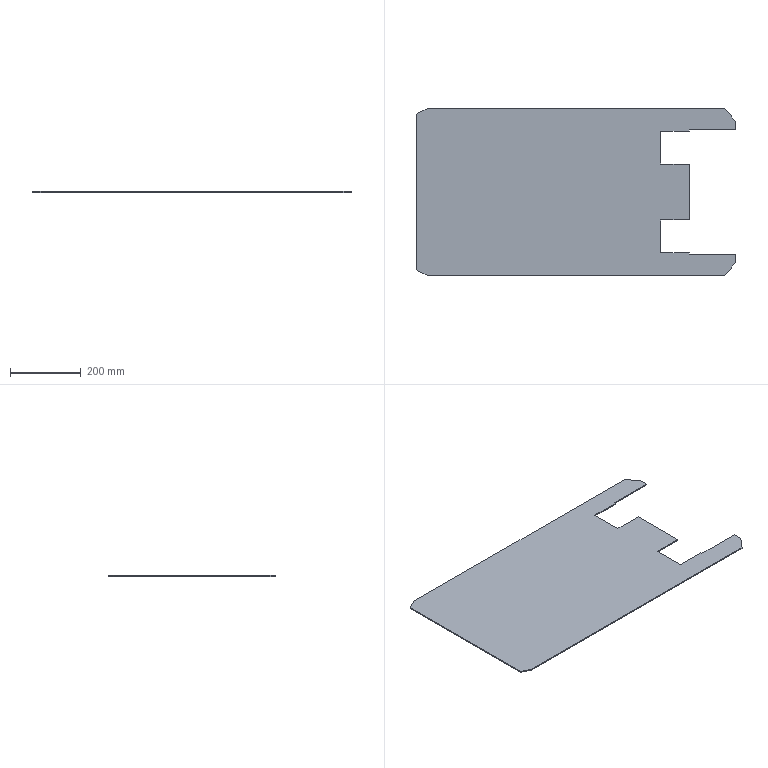Part | SolidWorks | features Extrusion 1, ICE 1 | 1 solid | 22 faces | box 900 x 470 x 3 mm | volume 1083288 mm3 | plane 22
STEP:
#1=CARTESIAN_POINT('',(150.,171.,-1.5));
#2=VERTEX_POINT('',#1);
#3=CARTESIAN_POINT('',(150.,171.,1.5));
#4=VERTEX_POINT('',#3);
#5=CARTESIAN_POINT('',(150.,171.,-1.5));
#6=DIRECTION('',(0.,0.,1.));
#7=VECTOR('',#6,1000.);
#8=LINE('',#5,#7);
#9=EDGE_CURVE('',#2,#4,#8,.T.);
#10=ORIENTED_EDGE('',*,*,#9,.F.);
#11=CARTESIAN_POINT('',(150.,175.,-1.5));
#12=VERTEX_POINT('',#11);
#13=CARTESIAN_POINT('',(150.,-175.,-1.5));
#14=DIRECTION('',(0.,1.,0.));
#15=VECTOR('',#14,1000.);
#16=LINE('',#13,#15);
#17=EDGE_CURVE('',#2,#12,#16,.T.);
#18=ORIENTED_EDGE('',*,*,#17,.T.);
#19=CARTESIAN_POINT('',(150.,175.,1.5));
#20=VERTEX_POINT('',#19);
#21=CARTESIAN_POINT('',(150.,175.,-1.5));
#22=DIRECTION('',(0.,0.,1.));
#23=VECTOR('',#22,1000.);
#24=LINE('',#21,#23);
#25=EDGE_CURVE('',#12,#20,#24,.T.);
#26=ORIENTED_EDGE('',*,*,#25,.T.);
#27=CARTESIAN_POINT('',(150.,-175.,1.5));
#28=DIRECTION('',(0.,1.,0.));
#29=VECTOR('',#28,1000.);
#30=LINE('',#27,#29);
#31=EDGE_CURVE('',#4,#20,#30,.T.);
#32=ORIENTED_EDGE('',*,*,#31,.F.);
#33=EDGE_LOOP('',(#10,#18,#26,#32));
#34=FACE_OUTER_BOUND('',#33,.T.);
#35=CARTESIAN_POINT('',(150.,-175.,-1.5));
#36=DIRECTION('',(1.,0.,0.));
#37=DIRECTION('',(0.,0.,-1.));
#38=AXIS2_PLACEMENT_3D('',#35,#36,#37);
#39=PLANE('',#38);
#40=ADVANCED_FACE('',(#34),#39,.T.);
#41=CARTESIAN_POINT('',(150.,79.,1.5));
#42=VERTEX_POINT('',#41);
#43=CARTESIAN_POINT('',(150.,79.,-1.5));
#44=VERTEX_POINT('',#43);
#45=CARTESIAN_POINT('',(150.,79.,-1.5));
#46=DIRECTION('',(0.,0.,-1.));
#47=VECTOR('',#46,1000.);
#48=LINE('',#45,#47);
#49=EDGE_CURVE('',#42,#44,#48,.T.);
#50=ORIENTED_EDGE('',*,*,#49,.F.);
#51=CARTESIAN_POINT('',(150.,-79.,1.5));
#52=VERTEX_POINT('',#51);
#53=CARTESIAN_POINT('',(150.,-175.,1.5));
#54=DIRECTION('',(0.,1.,0.));
#55=VECTOR('',#54,1000.);
#56=LINE('',#53,#55);
#57=EDGE_CURVE('',#52,#42,#56,.T.);
#58=ORIENTED_EDGE('',*,*,#57,.F.);
#59=CARTESIAN_POINT('',(150.,-79.,-1.5));
#60=VERTEX_POINT('',#59);
#61=CARTESIAN_POINT('',(150.,-79.,-1.5));
#62=DIRECTION('',(0.,0.,1.));
#63=VECTOR('',#62,1000.);
#64=LINE('',#61,#63);
#65=EDGE_CURVE('',#60,#52,#64,.T.);
#66=ORIENTED_EDGE('',*,*,#65,.F.);
#67=CARTESIAN_POINT('',(150.,-175.,-1.5));
#68=DIRECTION('',(0.,1.,0.));
#69=VECTOR('',#68,1000.);
#70=LINE('',#67,#69);
#71=EDGE_CURVE('',#60,#44,#70,.T.);
#72=ORIENTED_EDGE('',*,*,#71,.T.);
#73=EDGE_LOOP('',(#50,#58,#66,#72));
#74=FACE_OUTER_BOUND('',#73,.T.);
#75=CARTESIAN_POINT('',(150.,-175.,-1.5));
#76=DIRECTION('',(1.,0.,0.));
#77=DIRECTION('',(0.,0.,-1.));
#78=AXIS2_PLACEMENT_3D('',#75,#76,#77);
#79=PLANE('',#78);
#80=ADVANCED_FACE('',(#74),#79,.T.);
#81=CARTESIAN_POINT('',(-620.,220.,1.5));
#82=VERTEX_POINT('',#81);
#83=CARTESIAN_POINT('',(-620.,-220.,1.5));
#84=VERTEX_POINT('',#83);
#85=CARTESIAN_POINT('',(-620.,220.,1.5));
#86=DIRECTION('',(0.,-1.,0.));
#87=VECTOR('',#86,1000.);
#88=LINE('',#85,#87);
#89=EDGE_CURVE('',#82,#84,#88,.T.);
#90=ORIENTED_EDGE('',*,*,#89,.F.);
#91=CARTESIAN_POINT('',(-620.,220.,-1.5));
#92=VERTEX_POINT('',#91);
#93=CARTESIAN_POINT('',(-620.,220.,-1.5));
#94=DIRECTION('',(0.,0.,1.));
#95=VECTOR('',#94,1000.);
#96=LINE('',#93,#95);
#97=EDGE_CURVE('',#92,#82,#96,.T.);
#98=ORIENTED_EDGE('',*,*,#97,.F.);
#99=CARTESIAN_POINT('',(-620.,-220.,-1.5));
#100=VERTEX_POINT('',#99);
#101=CARTESIAN_POINT('',(-620.,220.,-1.5));
#102=DIRECTION('',(0.,-1.,0.));
#103=VECTOR('',#102,1000.);
#104=LINE('',#101,#103);
#105=EDGE_CURVE('',#92,#100,#104,.T.);
#106=ORIENTED_EDGE('',*,*,#105,.T.);
#107=CARTESIAN_POINT('',(-620.,-220.,-1.5));
#108=DIRECTION('',(0.,0.,1.));
#109=VECTOR('',#108,1000.);
#110=LINE('',#107,#109);
#111=EDGE_CURVE('',#100,#84,#110,.T.);
#112=ORIENTED_EDGE('',*,*,#111,.T.);
#113=EDGE_LOOP('',(#90,#98,#106,#112));
#114=FACE_OUTER_BOUND('',#113,.T.);
#115=CARTESIAN_POINT('',(-620.,220.,-1.5));
#116=DIRECTION('',(-1.,0.,0.));
#117=DIRECTION('',(0.,0.,1.));
#118=AXIS2_PLACEMENT_3D('',#115,#116,#117);
#119=PLANE('',#118);
#120=ADVANCED_FACE('',(#114),#119,.T.);
#121=CARTESIAN_POINT('',(-590.,235.,1.5));
#122=VERTEX_POINT('',#121);
#123=CARTESIAN_POINT('',(-590.,235.,1.5));
#124=DIRECTION('',(-0.8944,-0.4472,0.));
#125=VECTOR('',#124,1000.);
#126=LINE('',#123,#125);
#127=EDGE_CURVE('',#122,#82,#126,.T.);
#128=ORIENTED_EDGE('',*,*,#127,.F.);
#129=CARTESIAN_POINT('',(-590.,235.,-1.5));
#130=VERTEX_POINT('',#129);
#131=CARTESIAN_POINT('',(-590.,235.,-1.5));
#132=DIRECTION('',(0.,0.,1.));
#133=VECTOR('',#132,1000.);
#134=LINE('',#131,#133);
#135=EDGE_CURVE('',#130,#122,#134,.T.);
#136=ORIENTED_EDGE('',*,*,#135,.F.);
#137=CARTESIAN_POINT('',(-590.,235.,-1.5));
#138=DIRECTION('',(-0.8944,-0.4472,0.));
#139=VECTOR('',#138,1000.);
#140=LINE('',#137,#139);
#141=EDGE_CURVE('',#130,#92,#140,.T.);
#142=ORIENTED_EDGE('',*,*,#141,.T.);
#143=ORIENTED_EDGE('',*,*,#97,.T.);
#144=EDGE_LOOP('',(#128,#136,#142,#143));
#145=FACE_OUTER_BOUND('',#144,.T.);
#146=CARTESIAN_POINT('',(-590.,235.,-1.5));
#147=DIRECTION('',(-0.4472,0.8944,0.));
#148=DIRECTION('',(-0.8944,-0.4472,0.));
#149=AXIS2_PLACEMENT_3D('',#146,#147,#148);
#150=PLANE('',#149);
#151=ADVANCED_FACE('',(#145),#150,.T.);
#152=CARTESIAN_POINT('',(250.,235.,1.5));
#153=VERTEX_POINT('',#152);
#154=CARTESIAN_POINT('',(250.,235.,1.5));
#155=DIRECTION('',(-1.,0.,0.));
#156=VECTOR('',#155,1000.);
#157=LINE('',#154,#156);
#158=EDGE_CURVE('',#153,#122,#157,.T.);
#159=ORIENTED_EDGE('',*,*,#158,.F.);
#160=CARTESIAN_POINT('',(250.,235.,-1.5));
#161=VERTEX_POINT('',#160);
#162=CARTESIAN_POINT('',(250.,235.,-1.5));
#163=DIRECTION('',(0.,0.,1.));
#164=VECTOR('',#163,1000.);
#165=LINE('',#162,#164);
#166=EDGE_CURVE('',#161,#153,#165,.T.);
#167=ORIENTED_EDGE('',*,*,#166,.F.);
#168=CARTESIAN_POINT('',(250.,235.,-1.5));
#169=DIRECTION('',(-1.,0.,0.));
#170=VECTOR('',#169,1000.);
#171=LINE('',#168,#170);
#172=EDGE_CURVE('',#161,#130,#171,.T.);
#173=ORIENTED_EDGE('',*,*,#172,.T.);
#174=ORIENTED_EDGE('',*,*,#135,.T.);
#175=EDGE_LOOP('',(#159,#167,#173,#174));
#176=FACE_OUTER_BOUND('',#175,.T.);
#177=CARTESIAN_POINT('',(250.,235.,-1.5));
#178=DIRECTION('',(0.,1.,0.));
#179=DIRECTION('',(0.,0.,1.));
#180=AXIS2_PLACEMENT_3D('',#177,#178,#179);
#181=PLANE('',#180);
#182=ADVANCED_FACE('',(#176),#181,.T.);
#183=CARTESIAN_POINT('',(280.,200.,1.5));
#184=VERTEX_POINT('',#183);
#185=CARTESIAN_POINT('',(280.,200.,1.5));
#186=DIRECTION('',(-0.6508,0.7593,0.));
#187=VECTOR('',#186,1000.);
#188=LINE('',#185,#187);
#189=EDGE_CURVE('',#184,#153,#188,.T.);
#190=ORIENTED_EDGE('',*,*,#189,.F.);
#191=CARTESIAN_POINT('',(280.,200.,-1.5));
#192=VERTEX_POINT('',#191);
#193=CARTESIAN_POINT('',(280.,200.,-1.5));
#194=DIRECTION('',(0.,0.,1.));
#195=VECTOR('',#194,1000.);
#196=LINE('',#193,#195);
#197=EDGE_CURVE('',#192,#184,#196,.T.);
#198=ORIENTED_EDGE('',*,*,#197,.F.);
#199=CARTESIAN_POINT('',(280.,200.,-1.5));
#200=DIRECTION('',(-0.6508,0.7593,0.));
#201=VECTOR('',#200,1000.);
#202=LINE('',#199,#201);
#203=EDGE_CURVE('',#192,#161,#202,.T.);
#204=ORIENTED_EDGE('',*,*,#203,.T.);
#205=ORIENTED_EDGE('',*,*,#166,.T.);
#206=EDGE_LOOP('',(#190,#198,#204,#205));
#207=FACE_OUTER_BOUND('',#206,.T.);
#208=CARTESIAN_POINT('',(280.,200.,-1.5));
#209=DIRECTION('',(0.7593,0.6508,0.));
#210=DIRECTION('',(-0.6508,0.7593,0.));
#211=AXIS2_PLACEMENT_3D('',#208,#209,#210);
#212=PLANE('',#211);
#213=ADVANCED_FACE('',(#207),#212,.T.);
#214=CARTESIAN_POINT('',(280.,175.,1.5));
#215=VERTEX_POINT('',#214);
#216=CARTESIAN_POINT('',(280.,175.,1.5));
#217=DIRECTION('',(0.,1.,0.));
#218=VECTOR('',#217,1000.);
#219=LINE('',#216,#218);
#220=EDGE_CURVE('',#215,#184,#219,.T.);
#221=ORIENTED_EDGE('',*,*,#220,.F.);
#222=CARTESIAN_POINT('',(280.,175.,-1.5));
#223=VERTEX_POINT('',#222);
#224=CARTESIAN_POINT('',(280.,175.,-1.5));
#225=DIRECTION('',(0.,0.,1.));
#226=VECTOR('',#225,1000.);
#227=LINE('',#224,#226);
#228=EDGE_CURVE('',#223,#215,#227,.T.);
#229=ORIENTED_EDGE('',*,*,#228,.F.);
#230=CARTESIAN_POINT('',(280.,175.,-1.5));
#231=DIRECTION('',(0.,1.,0.));
#232=VECTOR('',#231,1000.);
#233=LINE('',#230,#232);
#234=EDGE_CURVE('',#223,#192,#233,.T.);
#235=ORIENTED_EDGE('',*,*,#234,.T.);
#236=ORIENTED_EDGE('',*,*,#197,.T.);
#237=EDGE_LOOP('',(#221,#229,#235,#236));
#238=FACE_OUTER_BOUND('',#237,.T.);
#239=CARTESIAN_POINT('',(280.,175.,-1.5));
#240=DIRECTION('',(1.,0.,0.));
#241=DIRECTION('',(0.,0.,-1.));
#242=AXIS2_PLACEMENT_3D('',#239,#240,#241);
#243=PLANE('',#242);
#244=ADVANCED_FACE('',(#238),#243,.T.);
#245=CARTESIAN_POINT('',(150.,175.,1.5));
#246=DIRECTION('',(1.,0.,0.));
#247=VECTOR('',#246,1000.);
#248=LINE('',#245,#247);
#249=EDGE_CURVE('',#20,#215,#248,.T.);
#250=ORIENTED_EDGE('',*,*,#249,.F.);
#251=ORIENTED_EDGE('',*,*,#25,.F.);
#252=CARTESIAN_POINT('',(150.,175.,-1.5));
#253=DIRECTION('',(1.,0.,0.));
#254=VECTOR('',#253,1000.);
#255=LINE('',#252,#254);
#256=EDGE_CURVE('',#12,#223,#255,.T.);
#257=ORIENTED_EDGE('',*,*,#256,.T.);
#258=ORIENTED_EDGE('',*,*,#228,.T.);
#259=EDGE_LOOP('',(#250,#251,#257,#258));
#260=FACE_OUTER_BOUND('',#259,.T.);
#261=CARTESIAN_POINT('',(150.,175.,-1.5));
#262=DIRECTION('',(0.,-1.,0.));
#263=DIRECTION('',(0.,0.,-1.));
#264=AXIS2_PLACEMENT_3D('',#261,#262,#263);
#265=PLANE('',#264);
#266=ADVANCED_FACE('',(#260),#265,.T.);
#267=CARTESIAN_POINT('',(150.,-171.,1.5));
#268=VERTEX_POINT('',#267);
#269=CARTESIAN_POINT('',(150.,-171.,-1.5));
#270=VERTEX_POINT('',#269);
#271=CARTESIAN_POINT('',(150.,-171.,-1.5));
#272=DIRECTION('',(0.,0.,-1.));
#273=VECTOR('',#272,1000.);
#274=LINE('',#271,#273);
#275=EDGE_CURVE('',#268,#270,#274,.T.);
#276=ORIENTED_EDGE('',*,*,#275,.F.);
#277=CARTESIAN_POINT('',(150.,-175.,1.5));
#278=VERTEX_POINT('',#277);
#279=CARTESIAN_POINT('',(150.,-175.,1.5));
#280=DIRECTION('',(0.,1.,0.));
#281=VECTOR('',#280,1000.);
#282=LINE('',#279,#281);
#283=EDGE_CURVE('',#278,#268,#282,.T.);
#284=ORIENTED_EDGE('',*,*,#283,.F.);
#285=CARTESIAN_POINT('',(150.,-175.,-1.5));
#286=VERTEX_POINT('',#285);
#287=CARTESIAN_POINT('',(150.,-175.,-1.5));
#288=DIRECTION('',(0.,0.,1.));
#289=VECTOR('',#288,1000.);
#290=LINE('',#287,#289);
#291=EDGE_CURVE('',#286,#278,#290,.T.);
#292=ORIENTED_EDGE('',*,*,#291,.F.);
#293=CARTESIAN_POINT('',(150.,-175.,-1.5));
#294=DIRECTION('',(0.,1.,0.));
#295=VECTOR('',#294,1000.);
#296=LINE('',#293,#295);
#297=EDGE_CURVE('',#286,#270,#296,.T.);
#298=ORIENTED_EDGE('',*,*,#297,.T.);
#299=EDGE_LOOP('',(#276,#284,#292,#298));
#300=FACE_OUTER_BOUND('',#299,.T.);
#301=CARTESIAN_POINT('',(150.,-175.,-1.5));
#302=DIRECTION('',(1.,0.,0.));
#303=DIRECTION('',(0.,0.,-1.));
#304=AXIS2_PLACEMENT_3D('',#301,#302,#303);
#305=PLANE('',#304);
#306=ADVANCED_FACE('',(#300),#305,.T.);
#307=CARTESIAN_POINT('',(280.,-175.,1.5));
#308=VERTEX_POINT('',#307);
#309=CARTESIAN_POINT('',(280.,-175.,1.5));
#310=DIRECTION('',(-1.,0.,0.));
#311=VECTOR('',#310,1000.);
#312=LINE('',#309,#311);
#313=EDGE_CURVE('',#308,#278,#312,.T.);
#314=ORIENTED_EDGE('',*,*,#313,.F.);
#315=CARTESIAN_POINT('',(280.,-175.,-1.5));
#316=VERTEX_POINT('',#315);
#317=CARTESIAN_POINT('',(280.,-175.,-1.5));
#318=DIRECTION('',(0.,0.,1.));
#319=VECTOR('',#318,1000.);
#320=LINE('',#317,#319);
#321=EDGE_CURVE('',#316,#308,#320,.T.);
#322=ORIENTED_EDGE('',*,*,#321,.F.);
#323=CARTESIAN_POINT('',(280.,-175.,-1.5));
#324=DIRECTION('',(-1.,0.,0.));
#325=VECTOR('',#324,1000.);
#326=LINE('',#323,#325);
#327=EDGE_CURVE('',#316,#286,#326,.T.);
#328=ORIENTED_EDGE('',*,*,#327,.T.);
#329=ORIENTED_EDGE('',*,*,#291,.T.);
#330=EDGE_LOOP('',(#314,#322,#328,#329));
#331=FACE_OUTER_BOUND('',#330,.T.);
#332=CARTESIAN_POINT('',(280.,-175.,-1.5));
#333=DIRECTION('',(0.,1.,0.));
#334=DIRECTION('',(0.,0.,1.));
#335=AXIS2_PLACEMENT_3D('',#332,#333,#334);
#336=PLANE('',#335);
#337=ADVANCED_FACE('',(#331),#336,.T.);
#338=CARTESIAN_POINT('',(280.,-200.,1.5));
#339=VERTEX_POINT('',#338);
#340=CARTESIAN_POINT('',(280.,-200.,1.5));
#341=DIRECTION('',(0.,1.,0.));
#342=VECTOR('',#341,1000.);
#343=LINE('',#340,#342);
#344=EDGE_CURVE('',#339,#308,#343,.T.);
#345=ORIENTED_EDGE('',*,*,#344,.F.);
#346=CARTESIAN_POINT('',(280.,-200.,-1.5));
#347=VERTEX_POINT('',#346);
#348=CARTESIAN_POINT('',(280.,-200.,-1.5));
#349=DIRECTION('',(0.,0.,1.));
#350=VECTOR('',#349,1000.);
#351=LINE('',#348,#350);
#352=EDGE_CURVE('',#347,#339,#351,.T.);
#353=ORIENTED_EDGE('',*,*,#352,.F.);
#354=CARTESIAN_POINT('',(280.,-200.,-1.5));
#355=DIRECTION('',(0.,1.,0.));
#356=VECTOR('',#355,1000.);
#357=LINE('',#354,#356);
#358=EDGE_CURVE('',#347,#316,#357,.T.);
#359=ORIENTED_EDGE('',*,*,#358,.T.);
#360=ORIENTED_EDGE('',*,*,#321,.T.);
#361=EDGE_LOOP('',(#345,#353,#359,#360));
#362=FACE_OUTER_BOUND('',#361,.T.);
#363=CARTESIAN_POINT('',(280.,-200.,-1.5));
#364=DIRECTION('',(1.,0.,0.));
#365=DIRECTION('',(0.,0.,-1.));
#366=AXIS2_PLACEMENT_3D('',#363,#364,#365);
#367=PLANE('',#366);
#368=ADVANCED_FACE('',(#362),#367,.T.);
#369=CARTESIAN_POINT('',(250.,-235.,1.5));
#370=VERTEX_POINT('',#369);
#371=CARTESIAN_POINT('',(250.,-235.,1.5));
#372=DIRECTION('',(0.6508,0.7593,0.));
#373=VECTOR('',#372,1000.);
#374=LINE('',#371,#373);
#375=EDGE_CURVE('',#370,#339,#374,.T.);
#376=ORIENTED_EDGE('',*,*,#375,.F.);
#377=CARTESIAN_POINT('',(250.,-235.,-1.5));
#378=VERTEX_POINT('',#377);
#379=CARTESIAN_POINT('',(250.,-235.,-1.5));
#380=DIRECTION('',(0.,0.,1.));
#381=VECTOR('',#380,1000.);
#382=LINE('',#379,#381);
#383=EDGE_CURVE('',#378,#370,#382,.T.);
#384=ORIENTED_EDGE('',*,*,#383,.F.);
#385=CARTESIAN_POINT('',(250.,-235.,-1.5));
#386=DIRECTION('',(0.6508,0.7593,0.));
#387=VECTOR('',#386,1000.);
#388=LINE('',#385,#387);
#389=EDGE_CURVE('',#378,#347,#388,.T.);
#390=ORIENTED_EDGE('',*,*,#389,.T.);
#391=ORIENTED_EDGE('',*,*,#352,.T.);
#392=EDGE_LOOP('',(#376,#384,#390,#391));
#393=FACE_OUTER_BOUND('',#392,.T.);
#394=CARTESIAN_POINT('',(250.,-235.,-1.5));
#395=DIRECTION('',(0.7593,-0.6508,0.));
#396=DIRECTION('',(0.6508,0.7593,0.));
#397=AXIS2_PLACEMENT_3D('',#394,#395,#396);
#398=PLANE('',#397);
#399=ADVANCED_FACE('',(#393),#398,.T.);
#400=CARTESIAN_POINT('',(-590.,-235.,1.5));
#401=VERTEX_POINT('',#400);
#402=CARTESIAN_POINT('',(-590.,-235.,1.5));
#403=DIRECTION('',(1.,0.,0.));
#404=VECTOR('',#403,1000.);
#405=LINE('',#402,#404);
#406=EDGE_CURVE('',#401,#370,#405,.T.);
#407=ORIENTED_EDGE('',*,*,#406,.F.);
#408=CARTESIAN_POINT('',(-590.,-235.,-1.5));
#409=VERTEX_POINT('',#408);
#410=CARTESIAN_POINT('',(-590.,-235.,-1.5));
#411=DIRECTION('',(0.,0.,1.));
#412=VECTOR('',#411,1000.);
#413=LINE('',#410,#412);
#414=EDGE_CURVE('',#409,#401,#413,.T.);
#415=ORIENTED_EDGE('',*,*,#414,.F.);
#416=CARTESIAN_POINT('',(-590.,-235.,-1.5));
#417=DIRECTION('',(1.,0.,0.));
#418=VECTOR('',#417,1000.);
#419=LINE('',#416,#418);
#420=EDGE_CURVE('',#409,#378,#419,.T.);
#421=ORIENTED_EDGE('',*,*,#420,.T.);
#422=ORIENTED_EDGE('',*,*,#383,.T.);
#423=EDGE_LOOP('',(#407,#415,#421,#422));
#424=FACE_OUTER_BOUND('',#423,.T.);
#425=CARTESIAN_POINT('',(-590.,-235.,-1.5));
#426=DIRECTION('',(0.,-1.,0.));
#427=DIRECTION('',(0.,0.,-1.));
#428=AXIS2_PLACEMENT_3D('',#425,#426,#427);
#429=PLANE('',#428);
#430=ADVANCED_FACE('',(#424),#429,.T.);
#431=CARTESIAN_POINT('',(-620.,-220.,1.5));
#432=DIRECTION('',(0.8944,-0.4472,0.));
#433=VECTOR('',#432,1000.);
#434=LINE('',#431,#433);
#435=EDGE_CURVE('',#84,#401,#434,.T.);
#436=ORIENTED_EDGE('',*,*,#435,.F.);
#437=ORIENTED_EDGE('',*,*,#111,.F.);
#438=CARTESIAN_POINT('',(-620.,-220.,-1.5));
#439=DIRECTION('',(0.8944,-0.4472,0.));
#440=VECTOR('',#439,1000.);
#441=LINE('',#438,#440);
#442=EDGE_CURVE('',#100,#409,#441,.T.);
#443=ORIENTED_EDGE('',*,*,#442,.T.);
#444=ORIENTED_EDGE('',*,*,#414,.T.);
#445=EDGE_LOOP('',(#436,#437,#443,#444));
#446=FACE_OUTER_BOUND('',#445,.T.);
#447=CARTESIAN_POINT('',(-620.,-220.,-1.5));
#448=DIRECTION('',(-0.4472,-0.8944,0.));
#449=DIRECTION('',(0.8944,-0.4472,0.));
#450=AXIS2_PLACEMENT_3D('',#447,#448,#449);
#451=PLANE('',#450);
#452=ADVANCED_FACE('',(#446),#451,.T.);
#453=ORIENTED_EDGE('',*,*,#17,.F.);
#454=CARTESIAN_POINT('',(69.,171.,-1.5));
#455=VERTEX_POINT('',#454);
#456=CARTESIAN_POINT('',(0.,171.,-1.5));
#457=DIRECTION('',(-1.,0.,0.));
#458=VECTOR('',#457,1000.);
#459=LINE('',#456,#458);
#460=EDGE_CURVE('',#2,#455,#459,.T.);
#461=ORIENTED_EDGE('',*,*,#460,.T.);
#462=CARTESIAN_POINT('',(69.,79.,-1.5));
#463=VERTEX_POINT('',#462);
#464=CARTESIAN_POINT('',(69.,0.,-1.5));
#465=DIRECTION('',(0.,-1.,0.));
#466=VECTOR('',#465,1000.);
#467=LINE('',#464,#466);
#468=EDGE_CURVE('',#455,#463,#467,.T.);
#469=ORIENTED_EDGE('',*,*,#468,.T.);
#470=CARTESIAN_POINT('',(0.,79.,-1.5));
#471=DIRECTION('',(1.,0.,0.));
#472=VECTOR('',#471,1000.);
#473=LINE('',#470,#472);
#474=EDGE_CURVE('',#463,#44,#473,.T.);
#475=ORIENTED_EDGE('',*,*,#474,.T.);
#476=ORIENTED_EDGE('',*,*,#71,.F.);
#477=CARTESIAN_POINT('',(69.,-79.,-1.5));
#478=VERTEX_POINT('',#477);
#479=CARTESIAN_POINT('',(0.,-79.,-1.5));
#480=DIRECTION('',(-1.,0.,0.));
#481=VECTOR('',#480,1000.);
#482=LINE('',#479,#481);
#483=EDGE_CURVE('',#60,#478,#482,.T.);
#484=ORIENTED_EDGE('',*,*,#483,.T.);
#485=CARTESIAN_POINT('',(69.,-171.,-1.5));
#486=VERTEX_POINT('',#485);
#487=CARTESIAN_POINT('',(69.,0.,-1.5));
#488=DIRECTION('',(0.,-1.,0.));
#489=VECTOR('',#488,1000.);
#490=LINE('',#487,#489);
#491=EDGE_CURVE('',#478,#486,#490,.T.);
#492=ORIENTED_EDGE('',*,*,#491,.T.);
#493=CARTESIAN_POINT('',(0.,-171.,-1.5));
#494=DIRECTION('',(1.,0.,0.));
#495=VECTOR('',#494,1000.);
#496=LINE('',#493,#495);
#497=EDGE_CURVE('',#486,#270,#496,.T.);
#498=ORIENTED_EDGE('',*,*,#497,.T.);
#499=ORIENTED_EDGE('',*,*,#297,.F.);
#500=ORIENTED_EDGE('',*,*,#327,.F.);
#501=ORIENTED_EDGE('',*,*,#358,.F.);
#502=ORIENTED_EDGE('',*,*,#389,.F.);
#503=ORIENTED_EDGE('',*,*,#420,.F.);
#504=ORIENTED_EDGE('',*,*,#442,.F.);
#505=ORIENTED_EDGE('',*,*,#105,.F.);
#506=ORIENTED_EDGE('',*,*,#141,.F.);
#507=ORIENTED_EDGE('',*,*,#172,.F.);
#508=ORIENTED_EDGE('',*,*,#203,.F.);
#509=ORIENTED_EDGE('',*,*,#234,.F.);
#510=ORIENTED_EDGE('',*,*,#256,.F.);
#511=EDGE_LOOP('',(#453,#461,#469,#475,#476,#484,#492,#498,#499,#500,#501,#502,#503,#504,#505,#506,#507,#508,#509,#510));
#512=FACE_OUTER_BOUND('',#511,.T.);
#513=CARTESIAN_POINT('',(0.,0.,-1.5));
#514=DIRECTION('',(0.,0.,1.));
#515=DIRECTION('',(1.,0.,0.));
#516=AXIS2_PLACEMENT_3D('',#513,#514,#515);
#517=PLANE('',#516);
#518=ADVANCED_FACE('',(#512),#517,.F.);
#519=CARTESIAN_POINT('',(69.,171.,1.5));
#520=VERTEX_POINT('',#519);
#521=CARTESIAN_POINT('',(0.,171.,1.5));
#522=DIRECTION('',(-1.,0.,0.));
#523=VECTOR('',#522,1000.);
#524=LINE('',#521,#523);
#525=EDGE_CURVE('',#4,#520,#524,.T.);
#526=ORIENTED_EDGE('',*,*,#525,.F.);
#527=ORIENTED_EDGE('',*,*,#31,.T.);
#528=ORIENTED_EDGE('',*,*,#249,.T.);
#529=ORIENTED_EDGE('',*,*,#220,.T.);
#530=ORIENTED_EDGE('',*,*,#189,.T.);
#531=ORIENTED_EDGE('',*,*,#158,.T.);
#532=ORIENTED_EDGE('',*,*,#127,.T.);
#533=ORIENTED_EDGE('',*,*,#89,.T.);
#534=ORIENTED_EDGE('',*,*,#435,.T.);
#535=ORIENTED_EDGE('',*,*,#406,.T.);
#536=ORIENTED_EDGE('',*,*,#375,.T.);
#537=ORIENTED_EDGE('',*,*,#344,.T.);
#538=ORIENTED_EDGE('',*,*,#313,.T.);
#539=ORIENTED_EDGE('',*,*,#283,.T.);
#540=CARTESIAN_POINT('',(69.,-171.,1.5));
#541=VERTEX_POINT('',#540);
#542=CARTESIAN_POINT('',(0.,-171.,1.5));
#543=DIRECTION('',(1.,0.,0.));
#544=VECTOR('',#543,1000.);
#545=LINE('',#542,#544);
#546=EDGE_CURVE('',#541,#268,#545,.T.);
#547=ORIENTED_EDGE('',*,*,#546,.F.);
#548=CARTESIAN_POINT('',(69.,-79.,1.5));
#549=VERTEX_POINT('',#548);
#550=CARTESIAN_POINT('',(69.,0.,1.5));
#551=DIRECTION('',(0.,-1.,0.));
#552=VECTOR('',#551,1000.);
#553=LINE('',#550,#552);
#554=EDGE_CURVE('',#549,#541,#553,.T.);
#555=ORIENTED_EDGE('',*,*,#554,.F.);
#556=CARTESIAN_POINT('',(0.,-79.,1.5));
#557=DIRECTION('',(-1.,0.,0.));
#558=VECTOR('',#557,1000.);
#559=LINE('',#556,#558);
#560=EDGE_CURVE('',#52,#549,#559,.T.);
#561=ORIENTED_EDGE('',*,*,#560,.F.);
#562=ORIENTED_EDGE('',*,*,#57,.T.);
#563=CARTESIAN_POINT('',(69.,79.,1.5));
#564=VERTEX_POINT('',#563);
#565=CARTESIAN_POINT('',(0.,79.,1.5));
#566=DIRECTION('',(1.,0.,0.));
#567=VECTOR('',#566,1000.);
#568=LINE('',#565,#567);
#569=EDGE_CURVE('',#564,#42,#568,.T.);
#570=ORIENTED_EDGE('',*,*,#569,.F.);
#571=CARTESIAN_POINT('',(69.,0.,1.5));
#572=DIRECTION('',(0.,-1.,0.));
#573=VECTOR('',#572,1000.);
#574=LINE('',#571,#573);
#575=EDGE_CURVE('',#520,#564,#574,.T.);
#576=ORIENTED_EDGE('',*,*,#575,.F.);
#577=EDGE_LOOP('',(#526,#527,#528,#529,#530,#531,#532,#533,#534,#535,#536,#537,#538,#539,#547,#555,#561,#562,#570,#576));
#578=FACE_OUTER_BOUND('',#577,.T.);
#579=CARTESIAN_POINT('',(0.,0.,1.5));
#580=DIRECTION('',(0.,0.,1.));
#581=DIRECTION('',(1.,0.,0.));
#582=AXIS2_PLACEMENT_3D('',#579,#580,#581);
#583=PLANE('',#582);
#584=ADVANCED_FACE('',(#578),#583,.T.);
#585=CARTESIAN_POINT('',(69.,-79.,-15.));
#586=DIRECTION('',(0.,0.,1.));
#587=VECTOR('',#586,1000.);
#588=LINE('',#585,#587);
#589=EDGE_CURVE('',#478,#549,#588,.T.);
#590=ORIENTED_EDGE('',*,*,#589,.T.);
#591=ORIENTED_EDGE('',*,*,#554,.T.);
#592=CARTESIAN_POINT('',(69.,-171.,-15.));
#593=DIRECTION('',(0.,0.,1.));
#594=VECTOR('',#593,1000.);
#595=LINE('',#592,#594);
#596=EDGE_CURVE('',#486,#541,#595,.T.);
#597=ORIENTED_EDGE('',*,*,#596,.F.);
#598=ORIENTED_EDGE('',*,*,#491,.F.);
#599=EDGE_LOOP('',(#590,#591,#597,#598));
#600=FACE_OUTER_BOUND('',#599,.T.);
#601=CARTESIAN_POINT('',(69.,-79.,-15.));
#602=DIRECTION('',(-1.,0.,0.));
#603=DIRECTION('',(0.,0.,1.));
#604=AXIS2_PLACEMENT_3D('',#601,#602,#603);
#605=PLANE('',#604);
#606=ADVANCED_FACE('',(#600),#605,.F.);
#607=ORIENTED_EDGE('',*,*,#65,.T.);
#608=ORIENTED_EDGE('',*,*,#560,.T.);
#609=ORIENTED_EDGE('',*,*,#589,.F.);
#610=ORIENTED_EDGE('',*,*,#483,.F.);
#611=EDGE_LOOP('',(#607,#608,#609,#610));
#612=FACE_OUTER_BOUND('',#611,.T.);
#613=CARTESIAN_POINT('',(171.,-79.,-15.));
#614=DIRECTION('',(0.,1.,0.));
#615=DIRECTION('',(0.,0.,1.));
#616=AXIS2_PLACEMENT_3D('',#613,#614,#615);
#617=PLANE('',#616);
#618=ADVANCED_FACE('',(#612),#617,.F.);
#619=ORIENTED_EDGE('',*,*,#596,.T.);
#620=ORIENTED_EDGE('',*,*,#546,.T.);
#621=ORIENTED_EDGE('',*,*,#275,.T.);
#622=ORIENTED_EDGE('',*,*,#497,.F.);
#623=EDGE_LOOP('',(#619,#620,#621,#622));
#624=FACE_OUTER_BOUND('',#623,.T.);
#625=CARTESIAN_POINT('',(69.,-171.,-15.));
#626=DIRECTION('',(0.,-1.,0.));
#627=DIRECTION('',(0.,0.,-1.));
#628=AXIS2_PLACEMENT_3D('',#625,#626,#627);
#629=PLANE('',#628);
#630=ADVANCED_FACE('',(#624),#629,.F.);
#631=CARTESIAN_POINT('',(69.,171.,-15.));
#632=DIRECTION('',(0.,0.,1.));
#633=VECTOR('',#632,1000.);
#634=LINE('',#631,#633);
#635=EDGE_CURVE('',#455,#520,#634,.T.);
#636=ORIENTED_EDGE('',*,*,#635,.T.);
#637=ORIENTED_EDGE('',*,*,#575,.T.);
#638=CARTESIAN_POINT('',(69.,79.,-15.));
#639=DIRECTION('',(0.,0.,1.));
#640=VECTOR('',#639,1000.);
#641=LINE('',#638,#640);
#642=EDGE_CURVE('',#463,#564,#641,.T.);
#643=ORIENTED_EDGE('',*,*,#642,.F.);
#644=ORIENTED_EDGE('',*,*,#468,.F.);
#645=EDGE_LOOP('',(#636,#637,#643,#644));
#646=FACE_OUTER_BOUND('',#645,.T.);
#647=CARTESIAN_POINT('',(69.,171.,-15.));
#648=DIRECTION('',(-1.,0.,0.));
#649=DIRECTION('',(0.,0.,1.));
#650=AXIS2_PLACEMENT_3D('',#647,#648,#649);
#651=PLANE('',#650);
#652=ADVANCED_FACE('',(#646),#651,.F.);
#653=ORIENTED_EDGE('',*,*,#9,.T.);
#654=ORIENTED_EDGE('',*,*,#525,.T.);
#655=ORIENTED_EDGE('',*,*,#635,.F.);
#656=ORIENTED_EDGE('',*,*,#460,.F.);
#657=EDGE_LOOP('',(#653,#654,#655,#656));
#658=FACE_OUTER_BOUND('',#657,.T.);
#659=CARTESIAN_POINT('',(171.,171.,-15.));
#660=DIRECTION('',(0.,1.,0.));
#661=DIRECTION('',(0.,0.,1.));
#662=AXIS2_PLACEMENT_3D('',#659,#660,#661);
#663=PLANE('',#662);
#664=ADVANCED_FACE('',(#658),#663,.F.);
#665=ORIENTED_EDGE('',*,*,#642,.T.);
#666=ORIENTED_EDGE('',*,*,#569,.T.);
#667=ORIENTED_EDGE('',*,*,#49,.T.);
#668=ORIENTED_EDGE('',*,*,#474,.F.);
#669=EDGE_LOOP('',(#665,#666,#667,#668));
#670=FACE_OUTER_BOUND('',#669,.T.);
#671=CARTESIAN_POINT('',(69.,79.,-15.));
#672=DIRECTION('',(0.,-1.,0.));
#673=DIRECTION('',(0.,0.,-1.));
#674=AXIS2_PLACEMENT_3D('',#671,#672,#673);
#675=PLANE('',#674);
#676=ADVANCED_FACE('',(#670),#675,.F.);
#677=CLOSED_SHELL('',(#40,#80,#120,#151,#182,#213,#244,#266,#306,#337,#368,#399,#430,#452,#518,#584,#606,#618,#630,#652,#664,#676));
#678=MANIFOLD_SOLID_BREP('',#677);
#679=CARTESIAN_POINT('',(0.,0.,0.));
#680=DIRECTION('',(0.,0.,1.));
#681=DIRECTION('',(1.,0.,0.));
#682=AXIS2_PLACEMENT_3D('',#679,#680,#681);
#683=(LENGTH_UNIT()NAMED_UNIT(*)SI_UNIT(.MILLI.,.METRE.));
#684=UNCERTAINTY_MEASURE_WITH_UNIT(LENGTH_MEASURE(0.00001),#683,'','');
#685=(NAMED_UNIT(*)PLANE_ANGLE_UNIT()SI_UNIT($,.RADIAN.));
#686=(NAMED_UNIT(*)SI_UNIT($,.STERADIAN.)SOLID_ANGLE_UNIT());
#687=(GEOMETRIC_REPRESENTATION_CONTEXT(3)GLOBAL_UNCERTAINTY_ASSIGNED_CONTEXT((#684))GLOBAL_UNIT_ASSIGNED_CONTEXT((#683,#685,#686))REPRESENTATION_CONTEXT('',''));
#688=ADVANCED_BREP_SHAPE_REPRESENTATION('',(#678,#682),#687);